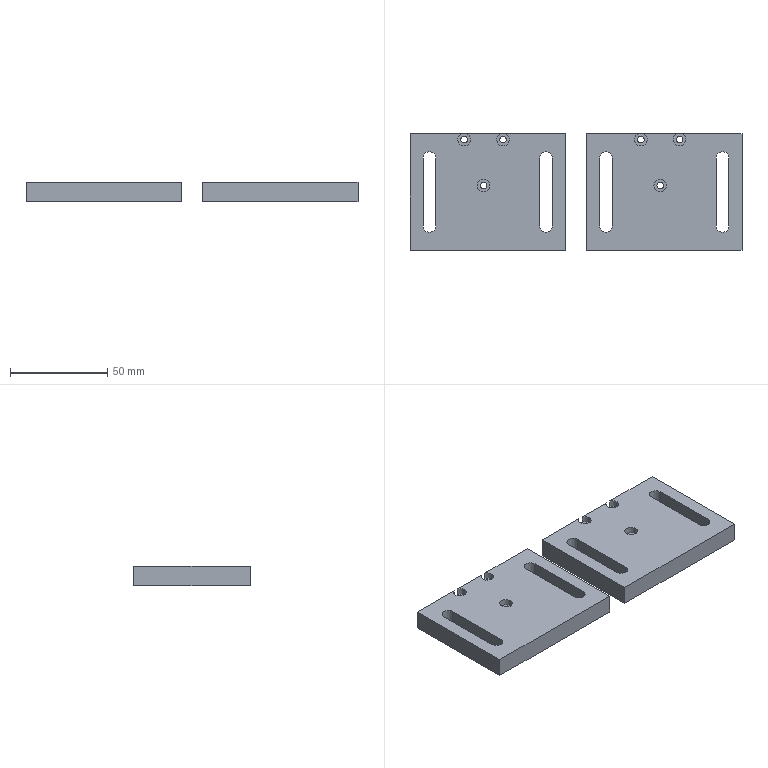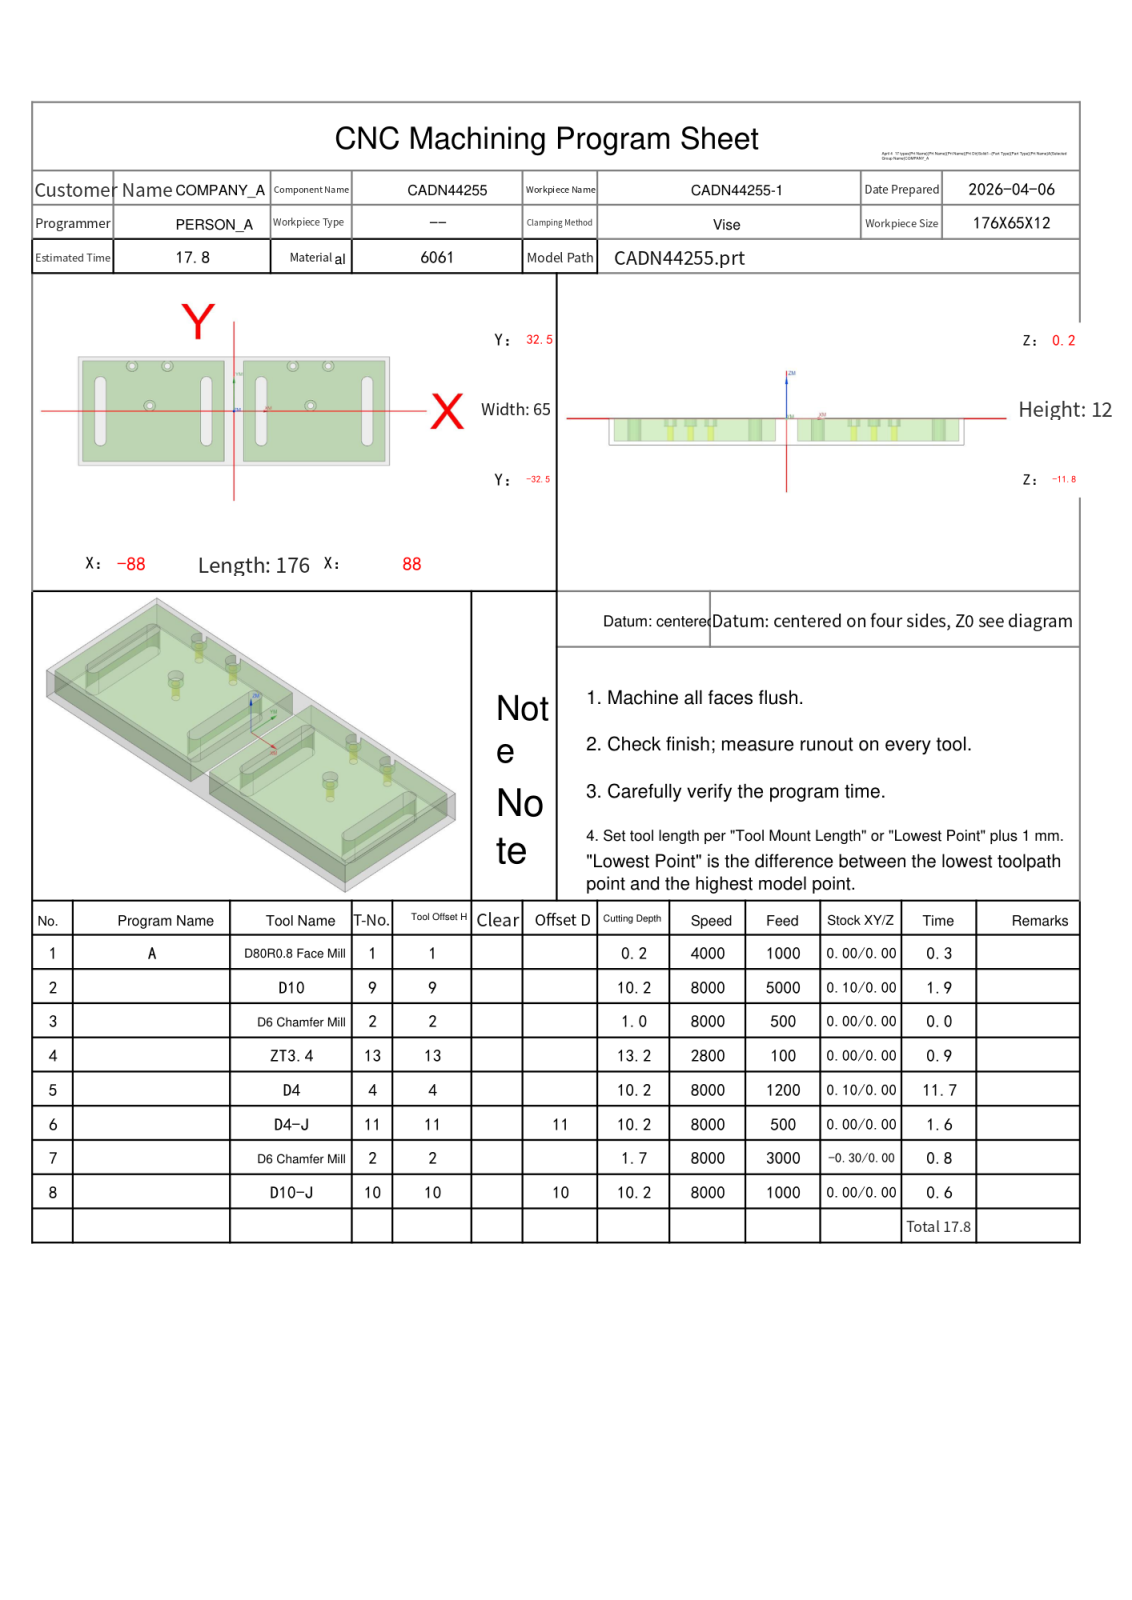NC program | NX | posted by the shop | part box 171 x 60 x 10 mm
Lines 1631 to 2411 of 2411:
N6 T11 M06
(D4-J  D=4. R=0. H=11 ce=0.00 di=0.00)
G00 G90 G54 X-37.607 Y27. M03 S8000
G43 H11 Z20.
M08
Z.5
G41 D11
G01 X-37.544 Y26.81 F500.
G03 X-36.966 Y26.391 I.579 J.19
X-36.357 Y27. I0.0 J.609
X-37.372 Y25.772 Z-3.4 I-1.25 J0.0
X-36.357 Y27. I-.234 J1.228
X-37.607 Y28.25 I-1.25 J0.0
X-38.857 Y27. I0.0 J-1.25
X-37.607 Y25.75 I1.25 J0.0
X-37.372 Y25.772 I0.0 J1.25
X-36.877 Y26.37 I-.114 J.598
X-37.408 Y26.974 I-.609 J0.0
G01 G40 X-37.607 Y27.
G00 Z20.
X-57.607
Z.5
G41 D11
G01 X-57.544 Y26.81
G03 X-56.966 Y26.391 I.579 J.19
X-56.357 Y27. I0.0 J.609
X-57.372 Y25.772 Z-3.4 I-1.25 J0.0
X-56.357 Y27. I-.234 J1.228
X-57.607 Y28.25 I-1.25 J0.0
X-58.857 Y27. I0.0 J-1.25
X-57.607 Y25.75 I1.25 J0.0
X-57.372 Y25.772 I0.0 J1.25
X-56.877 Y26.37 I-.114 J.598
X-57.408 Y26.974 I-.609 J0.0
G01 G40 X-57.607 Y27.
G00 Z20.
X-47.607 Y3.3
Z.5
G41 D11
G01 X-47.544 Y3.11
G03 X-46.966 Y2.691 I.579 J.19
X-46.357 Y3.3 I0.0 J.609
X-47.372 Y2.072 Z-3.4 I-1.25 J0.0
X-46.357 Y3.3 I-.234 J1.228
X-47.607 Y4.55 I-1.25 J0.0
X-48.857 Y3.3 I0.0 J-1.25
X-47.607 Y2.05 I1.25 J0.0
X-47.372 Y2.072 I0.0 J1.25
X-46.877 Y2.67 I-.114 J.598
X-47.408 Y3.274 I-.609 J0.0
G01 G40 X-47.607 Y3.3
G00 Z20.
X33.393 Y27.
Z.5
G41 D11
G01 X33.456 Y26.81
G03 X34.034 Y26.391 I.579 J.19
X34.643 Y27. I0.0 J.609
X33.628 Y25.772 Z-3.4 I-1.25 J0.0
X34.643 Y27. I-.234 J1.228
X33.393 Y28.25 I-1.25 J0.0
X32.143 Y27. I0.0 J-1.25
X33.393 Y25.75 I1.25 J0.0
X33.628 Y25.772 I0.0 J1.25
X34.123 Y26.37 I-.114 J.598
X33.592 Y26.974 I-.609 J0.0
G01 G40 X33.393 Y27.
G00 Z20.
X53.393
Z.5
G41 D11
G01 X53.456 Y26.81
G03 X54.034 Y26.391 I.579 J.19
X54.643 Y27. I0.0 J.609
X53.628 Y25.772 Z-3.4 I-1.25 J0.0
X54.643 Y27. I-.234 J1.228
X53.393 Y28.25 I-1.25 J0.0
X52.143 Y27. I0.0 J-1.25
X53.393 Y25.75 I1.25 J0.0
X53.628 Y25.772 I0.0 J1.25
X54.123 Y26.37 I-.114 J.598
X53.592 Y26.974 I-.609 J0.0
G01 G40 X53.393 Y27.
G00 Z20.
X43.393 Y3.3
Z.5
G41 D11
G01 X43.456 Y3.11
G03 X44.034 Y2.691 I.579 J.19
X44.643 Y3.3 I0.0 J.609
X43.628 Y2.072 Z-3.4 I-1.25 J0.0
X44.643 Y3.3 I-.234 J1.228
X43.393 Y4.55 I-1.25 J0.0
X42.143 Y3.3 I0.0 J-1.25
X43.393 Y2.05 I1.25 J0.0
X43.628 Y2.072 I0.0 J1.25
X44.123 Y2.67 I-.114 J.598
X43.592 Y3.274 I-.609 J0.0
G01 G40 X43.393 Y3.3
G00 Z20.
G00 G90 X76.5 Y-.2 M03 S6000
Z20.
Z-4.5
G01 Z-5. F500.
G41 D11
X76.55
G03 X76.75 Y0.0 I0.0 J.2
G01 Y17.5
G03 X75.5 Y18.75 I-1.25 J0.0
X74.25 Y17.5 I0.0 J-1.25
G01 Y-17.5
G03 X75.5 Y-18.75 I1.25 J0.0
X76.75 Y-17.5 I0.0 J1.25
G01 Y0.0
Y.5
G03 X76.55 Y.7 I-.2 J0.0
G01 G40 X76.5
Z-4.5
G00 Z1.
Y-.2
Z-9.5
G01 Z-10.
G41 D11
X76.55
G03 X76.75 Y0.0 I0.0 J.2
G01 Y17.5
G03 X75.5 Y18.75 I-1.25 J0.0
X74.25 Y17.5 I0.0 J-1.25
G01 Y-17.5
G03 X75.5 Y-18.75 I1.25 J0.0
X76.75 Y-17.5 I0.0 J1.25
G01 Y0.0
Y.5
G03 X76.55 Y.7 I-.2 J0.0
G01 G40 X76.5
Z-9.5
G00 Z20.
X16.5 Y-.2
Z-4.5
G01 Z-5.
G41 D11
X16.55
G03 X16.75 Y0.0 I0.0 J.2
G01 Y17.5
G03 X15.5 Y18.75 I-1.25 J0.0
X14.25 Y17.5 I0.0 J-1.25
G01 Y-17.5
G03 X15.5 Y-18.75 I1.25 J0.0
X16.75 Y-17.5 I0.0 J1.25
G01 Y0.0
Y.5
G03 X16.55 Y.7 I-.2 J0.0
G01 G40 X16.5
Z-4.5
G00 Z1.
Y-.2
Z-9.5
G01 Z-10.
G41 D11
X16.55
G03 X16.75 Y0.0 I0.0 J.2
G01 Y17.5
G03 X15.5 Y18.75 I-1.25 J0.0
X14.25 Y17.5 I0.0 J-1.25
G01 Y-17.5
G03 X15.5 Y-18.75 I1.25 J0.0
X16.75 Y-17.5 I0.0 J1.25
G01 Y0.0
Y.5
G03 X16.55 Y.7 I-.2 J0.0
G01 G40 X16.5
Z-9.5
G00 Z20.
X-14.5 Y-.2
Z-4.5
G01 Z-5.
G41 D11
X-14.45
G03 X-14.25 Y0.0 I0.0 J.2
G01 Y17.5
G03 X-15.5 Y18.75 I-1.25 J0.0
X-16.75 Y17.5 I0.0 J-1.25
G01 Y-17.5
G03 X-15.5 Y-18.75 I1.25 J0.0
X-14.25 Y-17.5 I0.0 J1.25
G01 Y0.0
Y.5
G03 X-14.45 Y.7 I-.2 J0.0
G01 G40 X-14.5
Z-4.5
G00 Z1.
Y-.2
Z-9.5
G01 Z-10.
G41 D11
X-14.45
G03 X-14.25 Y0.0 I0.0 J.2
G01 Y17.5
G03 X-15.5 Y18.75 I-1.25 J0.0
X-16.75 Y17.5 I0.0 J-1.25
G01 Y-17.5
G03 X-15.5 Y-18.75 I1.25 J0.0
X-14.25 Y-17.5 I0.0 J1.25
G01 Y0.0
Y.5
G03 X-14.45 Y.7 I-.2 J0.0
G01 G40 X-14.5
Z-9.5
G00 Z20.
X-76.5 Y.2
Z-4.5
G01 Z-5.
G41 D11
X-76.55
G03 X-76.75 Y0.0 I0.0 J-.2
G01 Y-17.5
G03 X-75.5 Y-18.75 I1.25 J0.0
X-74.25 Y-17.5 I0.0 J1.25
G01 Y17.5
G03 X-75.5 Y18.75 I-1.25 J0.0
X-76.75 Y17.5 I0.0 J-1.25
G01 Y0.0
Y-.5
G03 X-76.55 Y-.7 I.2 J0.0
G01 G40 X-76.5
Z-4.5
G00 Z1.
Y.2
Z-9.5
G01 Z-10.
G41 D11
X-76.55
G03 X-76.75 Y0.0 I0.0 J-.2
G01 Y-17.5
G03 X-75.5 Y-18.75 I1.25 J0.0
X-74.25 Y-17.5 I0.0 J1.25
G01 Y17.5
G03 X-75.5 Y18.75 I-1.25 J0.0
X-76.75 Y17.5 I0.0 J-1.25
G01 Y0.0
Y-.5
G03 X-76.55 Y-.7 I.2 J0.0
G01 G40 X-76.5
Z-9.5
G00 Z20.
G91 G28 Z0.0
M05
M09
G91 G28 Z0.0
M01
N7 T02 M06
(D6 Chamfer Mill  D=6. R=0. H=02 ce=0.00 di=0.00)
G00 G90 G54 X-45.25 Y-32.128 M03 S8000
G43 H02 Z20.
M08
Z2.099
G01 Z-1.5 F3000.
G03 X-45.17 Y-31.828 I-.52 J.3
X-45.47 Y-31.308 I-.6 J0.0
G01 X-45.5 Y-31.3
X-85.5
G02 X-86.8 Y-30. I0.0 J1.3
G01 Y30.
G02 X-85.5 Y31.3 I1.3 J0.0
G01 X-58.857
G02 X-57.607 Y30.357 I0.0 J-1.3
X-56.357 Y31.3 I1.25 J-.357
G01 X-38.857
G02 X-37.607 Y30.357 I0.0 J-1.3
X-36.357 Y31.3 I1.25 J-.357
G01 X-5.5
G02 X-4.2 Y30. I0.0 J-1.3
G01 Y-30.
G02 X-5.5 Y-31.3 I-1.3 J0.0
G01 X-45.5
X-45.53 Y-31.308
G03 X-45.83 Y-31.828 I.3 J-.52
X-45.75 Y-32.128 I.6 J0.0
G01 Z2.099
G00 Z20.
X-57.936 Y25.849
Z2.182
G01 Z-1.5
G03 X-57.989 Y25.602 I.546 J-.248
X-57.637 Y25.055 I.6 J0.0
G01 X-57.607 Y25.05
G03 X-55.657 Y27. I0.0 J1.95
X-55.983 Y28.081 I-1.95 J0.0
G01 X-56.225 Y28.376
X-56.52 Y28.619
X-56.857 Y28.8
X-57.111 Y28.941
X-57.328 Y29.136
X-57.496 Y29.374
X-57.607 Y29.643
X-57.717 Y29.374
X-57.885 Y29.136
X-58.102 Y28.941
X-58.357 Y28.8
G03 X-59.557 Y27. I.75 J-1.8
X-58.689 Y25.378 I1.95 J0.0
G01 X-58.352 Y25.198
X-57.987 Y25.087
X-57.607 Y25.05
X-57.576 Y25.055
G03 X-57.224 Y25.602 I-.248 J.546
X-57.277 Y25.849 I-.6 J0.0
G01 Z2.182
G00 Z20.
X-37.936
Z2.182
G01 Z-1.5
G03 X-37.989 Y25.602 I.546 J-.248
X-37.637 Y25.055 I.6 J0.0
G01 X-37.607 Y25.05
G03 X-35.657 Y27. I0.0 J1.95
X-35.983 Y28.081 I-1.95 J0.0
G01 X-36.225 Y28.376
X-36.52 Y28.619
X-36.857 Y28.8
X-37.111 Y28.941
X-37.328 Y29.136
X-37.496 Y29.374
X-37.607 Y29.643
X-37.717 Y29.374
X-37.885 Y29.136
X-38.102 Y28.941
X-38.357 Y28.8
G03 X-39.557 Y27. I.75 J-1.8
X-38.689 Y25.378 I1.95 J0.0
G01 X-38.352 Y25.198
X-37.987 Y25.087
X-37.607 Y25.05
X-37.576 Y25.055
G03 X-37.224 Y25.602 I-.248 J.546
X-37.277 Y25.849 I-.6 J0.0
G01 Z2.182
G00 Z20.
X-74.378 Y-.25
Z2.099
G01 Z-1.5
G03 X-74.078 Y-.33 I.3 J.52
X-73.558 Y-.03 I0.0 J.6
G01 X-73.55 Y0.0
Y17.5
G03 X-75.5 Y19.45 I-1.95 J0.0
X-77.45 Y17.5 I0.0 J-1.95
G01 Y-17.5
G03 X-75.5 Y-19.45 I1.95 J0.0
X-73.55 Y-17.5 I0.0 J1.95
G01 Y0.0
X-73.558 Y.03
G03 X-74.078 Y.33 I-.52 J-.3
X-74.378 Y.25 I0.0 J-.6
G01 Z2.099
G00 Z20.
X-16.622
Z2.099
G01 Z-1.5
G03 X-16.922 Y.33 I-.3 J-.52
X-17.442 Y.03 I0.0 J-.6
G01 X-17.45 Y0.0
Y-17.5
G03 X-15.5 Y-19.45 I1.95 J0.0
X-13.55 Y-17.5 I0.0 J1.95
G01 Y17.5
G03 X-15.5 Y19.45 I-1.95 J0.0
X-17.45 Y17.5 I0.0 J-1.95
G01 Y0.0
X-17.442 Y-.03
G03 X-16.922 Y-.33 I.52 J.3
X-16.622 Y-.25 I0.0 J.6
G01 Z2.099
G00 Z20.
X45.75 Y-32.128
Z2.099
G01 Z-1.5
G03 X45.83 Y-31.828 I-.52 J.3
X45.53 Y-31.308 I-.6 J0.0
G01 X45.5 Y-31.3
X5.5
G02 X4.2 Y-30. I0.0 J1.3
G01 Y30.
G02 X5.5 Y31.3 I1.3 J0.0
G01 X32.143
G02 X33.393 Y30.357 I0.0 J-1.3
X34.643 Y31.3 I1.25 J-.357
G01 X52.143
G02 X53.393 Y30.357 I0.0 J-1.3
X54.643 Y31.3 I1.25 J-.357
G01 X85.5
G02 X86.8 Y30. I0.0 J-1.3
G01 Y-30.
G02 X85.5 Y-31.3 I-1.3 J0.0
G01 X45.5
X45.47 Y-31.308
G03 X45.17 Y-31.828 I.3 J-.52
X45.25 Y-32.128 I.6 J0.0
G01 Z2.099
G00 Z20.
X33.064 Y25.849
Z2.182
G01 Z-1.5
G03 X33.011 Y25.602 I.546 J-.248
X33.363 Y25.055 I.6 J0.0
G01 X33.393 Y25.05
G03 X35.343 Y27. I0.0 J1.95
X35.017 Y28.081 I-1.95 J0.0
G01 X34.775 Y28.376
X34.48 Y28.619
X34.143 Y28.8
X33.889 Y28.941
X33.672 Y29.136
X33.504 Y29.374
X33.393 Y29.643
X33.283 Y29.374
X33.115 Y29.136
X32.898 Y28.941
X32.643 Y28.8
G03 X31.443 Y27. I.75 J-1.8
X32.311 Y25.378 I1.95 J0.0
G01 X32.648 Y25.198
X33.013 Y25.087
X33.393 Y25.05
X33.424 Y25.055
G03 X33.776 Y25.602 I-.248 J.546
X33.723 Y25.849 I-.6 J0.0
G01 Z2.182
G00 Z20.
X53.064
Z2.182
G01 Z-1.5
G03 X53.011 Y25.602 I.546 J-.248
X53.363 Y25.055 I.6 J0.0
G01 X53.393 Y25.05
G03 X55.343 Y27. I0.0 J1.95
X55.017 Y28.081 I-1.95 J0.0
G01 X54.775 Y28.376
X54.48 Y28.619
X54.143 Y28.8
X53.889 Y28.941
X53.672 Y29.136
X53.504 Y29.374
X53.393 Y29.643
X53.283 Y29.374
X53.115 Y29.136
X52.898 Y28.941
X52.643 Y28.8
G03 X51.443 Y27. I.75 J-1.8
X52.311 Y25.378 I1.95 J0.0
G01 X52.648 Y25.198
X53.013 Y25.087
X53.393 Y25.05
X53.424 Y25.055
G03 X53.776 Y25.602 I-.248 J.546
X53.723 Y25.849 I-.6 J0.0
G01 Z2.182
G00 Z20.
X16.622 Y-.25
Z2.099
G01 Z-1.5
G03 X16.922 Y-.33 I.3 J.52
X17.442 Y-.03 I0.0 J.6
G01 X17.45 Y0.0
Y17.5
G03 X15.5 Y19.45 I-1.95 J0.0
X13.55 Y17.5 I0.0 J-1.95
G01 Y-17.5
G03 X15.5 Y-19.45 I1.95 J0.0
X17.45 Y-17.5 I0.0 J1.95
G01 Y0.0
X17.442 Y.03
G03 X16.922 Y.33 I-.52 J-.3
X16.622 Y.25 I0.0 J-.6
G01 Z2.099
G00 Z20.
X74.378
Z2.099
G01 Z-1.5
G03 X74.078 Y.33 I-.3 J-.52
X73.558 Y.03 I0.0 J-.6
G01 X73.55 Y0.0
Y-17.5
G03 X75.5 Y-19.45 I1.95 J0.0
X77.45 Y-17.5 I0.0 J1.95
G01 Y17.5
G03 X75.5 Y19.45 I-1.95 J0.0
X73.55 Y17.5 I0.0 J-1.95
G01 Y0.0
X73.558 Y-.03
G03 X74.078 Y-.33 I.52 J.3
X74.378 Y-.25 I0.0 J.6
G01 Z2.099
G00 Z20.
G00 G90 X-45.543 Y1.803 M03 S8000
Z20.
Z2.5
G01 X-45.498 Y1.86 Z2.474 F500.
X-45.326 Y2.153 Z2.35
X-45.194 Y2.466 Z2.226
X-45.104 Y2.793 Z2.103
X-45.059 Y3.13 Z1.979
Y3.47 Z1.855
X-45.104 Y3.807 Z1.732
X-45.194 Y4.134 Z1.608
X-45.326 Y4.447 Z1.484
X-45.498 Y4.74 Z1.361
X-45.708 Y5.007 Z1.237
X-45.952 Y5.244 Z1.113
X-46.224 Y5.447 Z.99
X-46.439 Y5.57 Z.9
X-46.75 Y5.705 Z.776
X-47.077 Y5.798 Z.652
X-47.414 Y5.846 Z.529
X-47.753 Y5.849 Z.405
X-48.09 Y5.807 Z.281
X-48.419 Y5.72 Z.158
X-48.733 Y5.591 Z.034
X-49.027 Y5.421 Z-.089
X-49.296 Y5.214 Z-.213
X-49.535 Y4.972 Z-.337
X-49.74 Y4.702 Z-.46
X-49.908 Y4.406 Z-.584
X-50.034 Y4.09 Z-.708
X-50.118 Y3.761 Z-.831
X-50.157 Y3.424 Z-.955
Y3.3 Z-1.
G03 X-47.607 Y.75 I2.55 J0.0
X-45.057 Y3.3 I0.0 J2.55
X-47.607 Y5.85 I-2.55 J0.0
X-50.157 Y3.3 I0.0 J-2.55
X-50.108 Y2.803 I2.55 J0.0
G01 Z1.5
G00 Z20.
X-59.846 Y25.787
Z2.5
G01 X-59.763 Y25.633 Z2.436
X-59.556 Y25.352 Z2.309
X-59.313 Y25.101 Z2.182
X-59.038 Y24.886 Z2.055
X-58.737 Y24.711 Z1.928
X-58.414 Y24.578 Z1.801
X-58.077 Y24.491 Z1.674
X-57.73 Y24.45 Z1.547
X-57.483 Z1.457
X-57.136 Y24.491 Z1.33
X-56.799 Y24.578 Z1.203
X-56.476 Y24.711 Z1.076
X-56.175 Y24.886 Z.95
X-55.9 Y25.101 Z.823
X-55.657 Y25.352 Z.696
X-55.45 Y25.633 Z.569
X-55.284 Y25.94 Z.442
X-55.161 Y26.266 Z.315
X-55.084 Y26.606 Z.188
X-55.054 Y26.954 Z.061
X-55.071 Y27.302 Z-.066
X-55.136 Y27.645 Z-.193
X-55.247 Y27.976 Z-.32
X-55.402 Y28.288 Z-.447
X-55.598 Y28.577 Z-.574
X-55.832 Y28.836 Z-.701
X-56.099 Y29.06 Z-.828
X-56.394 Y29.247 Z-.955
X-56.505 Y29.3 Z-1.
X-58.708
G03 X-60.157 Y27. I1.101 J-2.3
X-57.607 Y24.45 I2.55 J0.0
X-55.057 Y27. I0.0 J2.55
X-56.505 Y29.3 I-2.55 J0.0
G01 X-57.005
Z1.5
G00 Z20.
X-39.846 Y25.787
Z2.5
G01 X-39.763 Y25.633 Z2.436
X-39.556 Y25.352 Z2.309
X-39.313 Y25.101 Z2.182
X-39.038 Y24.886 Z2.055
X-38.737 Y24.711 Z1.928
X-38.414 Y24.578 Z1.801
X-38.077 Y24.491 Z1.674
X-37.73 Y24.45 Z1.547
X-37.483 Z1.457
X-37.136 Y24.491 Z1.33
X-36.799 Y24.578 Z1.203
X-36.476 Y24.711 Z1.076
X-36.175 Y24.886 Z.95
X-35.9 Y25.101 Z.823
X-35.657 Y25.352 Z.696
X-35.45 Y25.633 Z.569
X-35.284 Y25.94 Z.442
X-35.161 Y26.266 Z.315
X-35.084 Y26.606 Z.188
X-35.054 Y26.954 Z.061
X-35.071 Y27.302 Z-.066
X-35.136 Y27.645 Z-.193
X-35.247 Y27.976 Z-.32
X-35.402 Y28.288 Z-.447
X-35.598 Y28.577 Z-.574
X-35.832 Y28.836 Z-.701
X-36.099 Y29.06 Z-.828
X-36.394 Y29.247 Z-.955
X-36.505 Y29.3 Z-1.
X-38.708
G03 X-40.157 Y27. I1.101 J-2.3
X-37.607 Y24.45 I2.55 J0.0
X-35.057 Y27. I0.0 J2.55
X-36.505 Y29.3 I-2.55 J0.0
G01 X-37.005
Z1.5
G00 Z20.
X31.154 Y25.787
Z2.5
G01 X31.237 Y25.633 Z2.436
X31.444 Y25.352 Z2.309
X31.687 Y25.101 Z2.182
X31.962 Y24.886 Z2.055
X32.263 Y24.711 Z1.928
X32.586 Y24.578 Z1.801
X32.923 Y24.491 Z1.674
X33.27 Y24.45 Z1.547
X33.517 Z1.457
X33.864 Y24.491 Z1.33
X34.201 Y24.578 Z1.203
X34.524 Y24.711 Z1.076
X34.825 Y24.886 Z.95
X35.1 Y25.101 Z.823
X35.343 Y25.352 Z.696
X35.55 Y25.633 Z.569
X35.716 Y25.94 Z.442
X35.839 Y26.266 Z.315
X35.916 Y26.606 Z.188
X35.946 Y26.954 Z.061
X35.929 Y27.302 Z-.066
X35.864 Y27.645 Z-.193
X35.753 Y27.976 Z-.32
X35.598 Y28.288 Z-.447
X35.402 Y28.577 Z-.574
X35.168 Y28.836 Z-.701
X34.901 Y29.06 Z-.828
X34.606 Y29.247 Z-.955
X34.495 Y29.3 Z-1.
X32.292
G03 X30.843 Y27. I1.101 J-2.3
X33.393 Y24.45 I2.55 J0.0
X35.943 Y27. I0.0 J2.55
X34.495 Y29.3 I-2.55 J0.0
G01 X33.995
Z1.5
G00 Z20.
X51.154 Y25.787
Z2.5
G01 X51.237 Y25.633 Z2.436
X51.444 Y25.352 Z2.309
X51.687 Y25.101 Z2.182
X51.962 Y24.886 Z2.055
X52.263 Y24.711 Z1.928
X52.586 Y24.578 Z1.801
X52.923 Y24.491 Z1.674
X53.27 Y24.45 Z1.547
X53.517 Z1.457
X53.864 Y24.491 Z1.33
X54.201 Y24.578 Z1.203
X54.524 Y24.711 Z1.076
X54.825 Y24.886 Z.95
X55.1 Y25.101 Z.823
X55.343 Y25.352 Z.696
X55.55 Y25.633 Z.569
X55.716 Y25.94 Z.442
X55.839 Y26.266 Z.315
X55.916 Y26.606 Z.188
X55.946 Y26.954 Z.061
X55.929 Y27.302 Z-.066
X55.864 Y27.645 Z-.193
X55.753 Y27.976 Z-.32
X55.598 Y28.288 Z-.447
X55.402 Y28.577 Z-.574
X55.168 Y28.836 Z-.701
X54.901 Y29.06 Z-.828
X54.606 Y29.247 Z-.955
X54.495 Y29.3 Z-1.
X52.292
G03 X50.843 Y27. I1.101 J-2.3
X53.393 Y24.45 I2.55 J0.0
X55.943 Y27. I0.0 J2.55
X54.495 Y29.3 I-2.55 J0.0
G01 X53.995
Z1.5
G00 Z20.
X45.457 Y1.803
Z2.5
G01 X45.502 Y1.86 Z2.474
X45.674 Y2.153 Z2.35
X45.806 Y2.466 Z2.226
X45.896 Y2.793 Z2.103
X45.941 Y3.13 Z1.979
Y3.47 Z1.855
X45.896 Y3.807 Z1.732
X45.806 Y4.134 Z1.608
X45.674 Y4.447 Z1.484
X45.502 Y4.74 Z1.361
X45.292 Y5.007 Z1.237
X45.048 Y5.244 Z1.113
X44.776 Y5.447 Z.99
X44.561 Y5.57 Z.9
X44.25 Y5.705 Z.776
X43.923 Y5.798 Z.652
X43.586 Y5.846 Z.529
X43.247 Y5.849 Z.405
X42.91 Y5.807 Z.281
X42.581 Y5.72 Z.158
X42.267 Y5.591 Z.034
X41.973 Y5.421 Z-.089
X41.704 Y5.214 Z-.213
X41.465 Y4.972 Z-.337
X41.26 Y4.702 Z-.46
X41.092 Y4.406 Z-.584
X40.966 Y4.09 Z-.708
X40.882 Y3.761 Z-.831
X40.843 Y3.424 Z-.955
Y3.3 Z-1.
G03 X43.393 Y.75 I2.55 J0.0
X45.943 Y3.3 I0.0 J2.55
X43.393 Y5.85 I-2.55 J0.0
X40.843 Y3.3 I0.0 J-2.55
X40.892 Y2.803 I2.55 J0.0
G01 Z1.5
G00 Z20.
G91 G28 Z0.0
M05
M09
G91 G28 Z0.0
M01
N8 T10 M06
(D10-J  D=10. R=0. H=10 ce=0.00 di=0.00)
G00 G90 G54 X-4.487 Y-36.116 M03 S8000
G43 H10 Z20.
M08
Z-9.5
G01 Z-10. F1000.
G41 D10
X-4.503 Y-35.917
G03 X-5.5 Y-35. I-.997 J-.083
G01 X-85.5
G02 X-90.5 Y-30. I0.0 J5.
G01 Y30.
G02 X-85.5 Y35. I5. J0.0
G01 X-5.5
G02 X-.5 Y30. I0.0 J-5.
G01 Y-30.
G02 X-5.5 Y-35. I-5. J0.0
G01 X-6.
G03 X-7. Y-36. I0.0 J-1.
G01 G40 Y-36.2
X.351 Y-33.453
G41 D10
X.526 Y-33.356
G03 X1.038 Y-32.483 I-.488 J.873
X.948 Y-32.069 I-1. J0.0
G02 X.5 Y-30. I4.552 J2.069
G01 Y30.
G02 X5.5 Y35. I5. J0.0
G01 X85.5
G02 X90.5 Y30. I0.0 J-5.
G01 Y-30.
G02 X85.5 Y-35. I-5. J0.0
G01 X5.5
G02 X.948 Y-32.069 I0.0 J5.
X.764 Y-31.604 I4.552 J2.069
G03 X-.183 Y-30.925 I-.947 J-.321
X-.504 Y-30.978 I0.0 J-1.
G01 G40 X0.0 Y-32.398
Z-9.5
G00 Z20.
M05
M09
G91 G28 Z0.0
G91 G28 Y0.0
M30
%